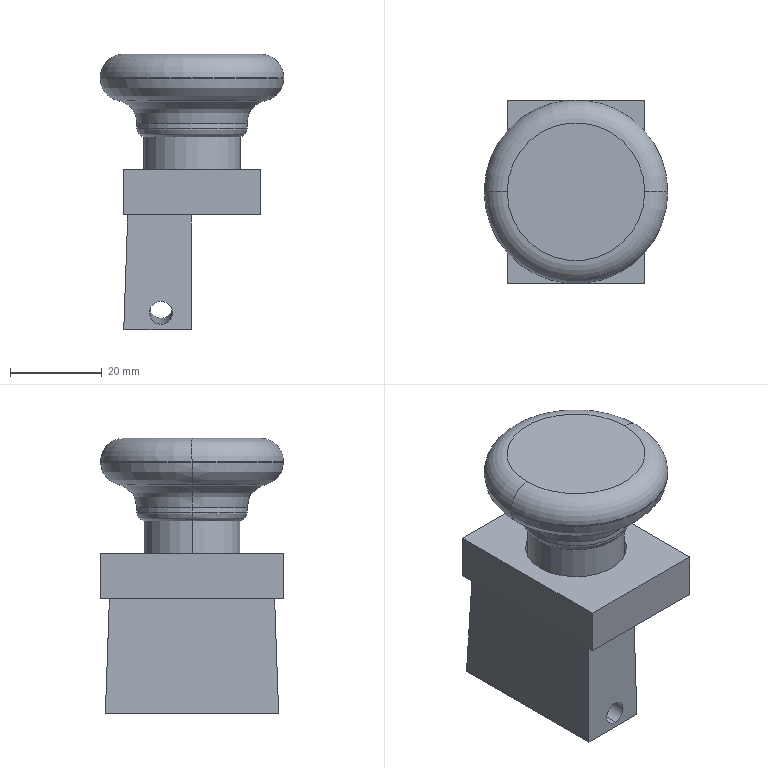Part | STEP file | PX950 (w)2) | 1 solid | 46 faces | box 40 x 40 x 60 mm | volume 29605 mm3 | plane 22 | cylinder 16 | torus 8 | commonest cylinder face diameters 22 x4 24 x4 5 x2 19 x2 21 x2 40 x2